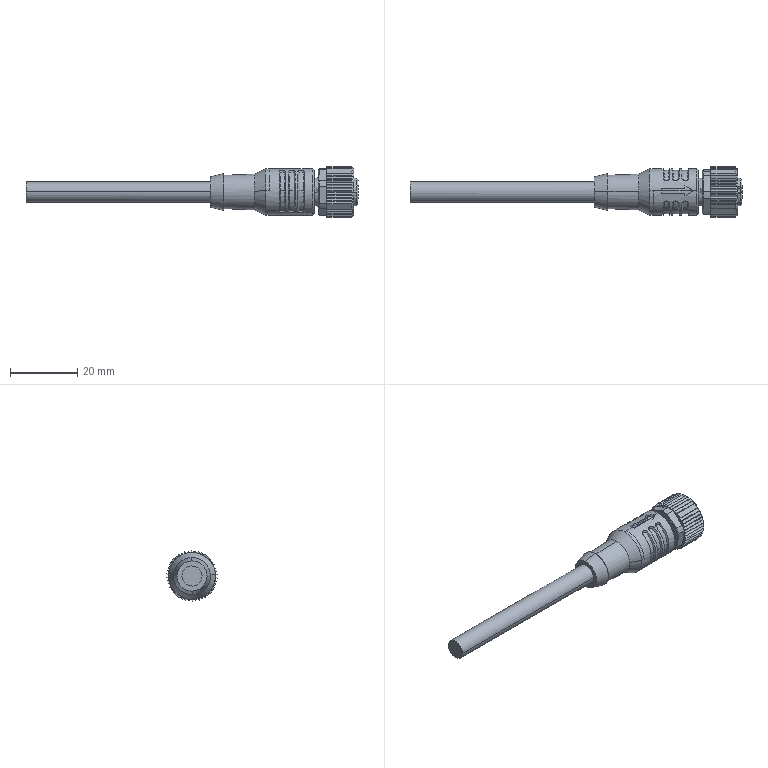Part | STEP file | BZJ-LSX-RGX M8分配器电缆6端口8芯Vertical出线3米(PVC)64S423-030 | 5 solids | 564 faces | box 99 x 14.979 x 14.996 mm | volume 5984 mm3 | spline 561 | cylinder 2 | plane 1 | commonest cylinder face diameters 4 x2